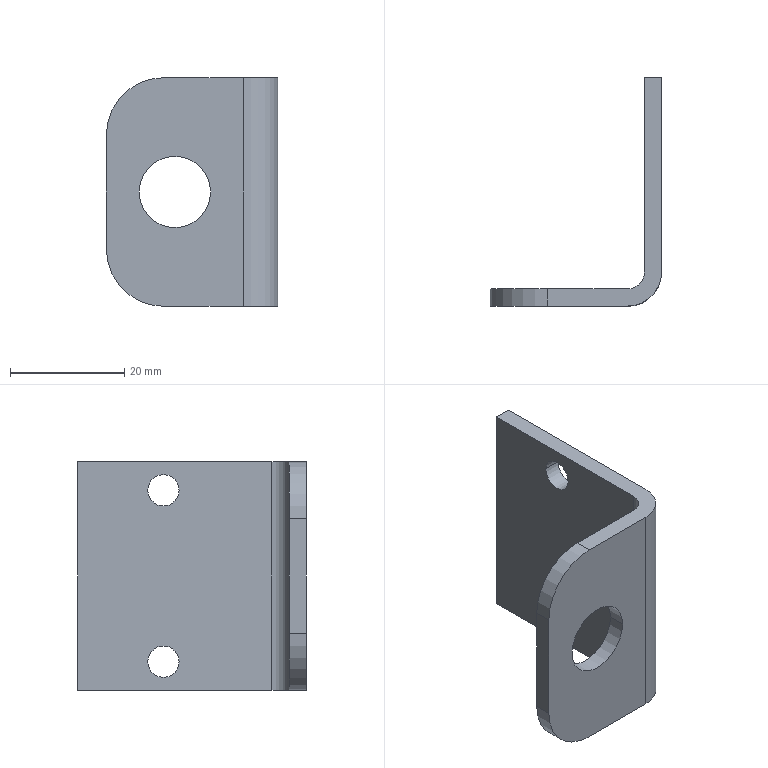Part | STEP file | X77-03025 | 1 solid | 18 faces | box 30 x 40 x 40 mm | volume 7169 mm3 | cylinder 10 | plane 8 | commonest cylinder face diameters 5.5 x4 12.5 x2 20 x2 6 x1 12 x1
STEP:
#1=CARTESIAN_POINT('',(-8.75,-40.,20.));
#2=VERTEX_POINT('',#1);
#3=CARTESIAN_POINT('',(-21.25,-40.,20.));
#4=VERTEX_POINT('',#3);
#5=CARTESIAN_POINT('',(-15.,-40.,20.));
#6=DIRECTION('',(0.,1.,0.));
#7=DIRECTION('',(-1.,0.,0.));
#8=AXIS2_PLACEMENT_3D('',#5,#6,#7);
#9=CIRCLE('',#8,6.25);
#10=EDGE_CURVE('',#2,#4,#9,.T.);
#11=ORIENTED_EDGE('',*,*,#10,.F.);
#12=CARTESIAN_POINT('',(-8.75,-37.,20.));
#13=VERTEX_POINT('',#12);
#14=CARTESIAN_POINT('',(-8.75,-40.,20.));
#15=DIRECTION('',(0.,1.,0.));
#16=VECTOR('',#15,1000.);
#17=LINE('',#14,#16);
#18=EDGE_CURVE('',#2,#13,#17,.T.);
#19=ORIENTED_EDGE('',*,*,#18,.T.);
#20=CARTESIAN_POINT('',(-21.25,-37.,20.));
#21=VERTEX_POINT('',#20);
#22=CARTESIAN_POINT('',(-15.,-37.,20.));
#23=DIRECTION('',(0.,1.,0.));
#24=DIRECTION('',(-1.,0.,0.));
#25=AXIS2_PLACEMENT_3D('',#22,#23,#24);
#26=CIRCLE('',#25,6.25);
#27=EDGE_CURVE('',#13,#21,#26,.T.);
#28=ORIENTED_EDGE('',*,*,#27,.T.);
#29=CARTESIAN_POINT('',(-21.25,-40.,20.));
#30=DIRECTION('',(0.,1.,0.));
#31=VECTOR('',#30,1000.);
#32=LINE('',#29,#31);
#33=EDGE_CURVE('',#4,#21,#32,.T.);
#34=ORIENTED_EDGE('',*,*,#33,.F.);
#35=EDGE_LOOP('',(#11,#19,#28,#34));
#36=FACE_OUTER_BOUND('',#35,.T.);
#37=CARTESIAN_POINT('',(-15.,-40.,20.));
#38=DIRECTION('',(0.,1.,0.));
#39=DIRECTION('',(-1.,0.,0.));
#40=AXIS2_PLACEMENT_3D('',#37,#38,#39);
#41=CYLINDRICAL_SURFACE('',#40,6.25);
#42=ADVANCED_FACE('',(#36),#41,.F.);
#43=CARTESIAN_POINT('',(3.,-12.25,35.));
#44=VERTEX_POINT('',#43);
#45=CARTESIAN_POINT('',(3.,-17.75,35.));
#46=VERTEX_POINT('',#45);
#47=CARTESIAN_POINT('',(3.,-15.,35.));
#48=DIRECTION('',(-1.,0.,0.));
#49=DIRECTION('',(0.,-1.,0.));
#50=AXIS2_PLACEMENT_3D('',#47,#48,#49);
#51=CIRCLE('',#50,2.75);
#52=EDGE_CURVE('',#44,#46,#51,.T.);
#53=ORIENTED_EDGE('',*,*,#52,.F.);
#54=CARTESIAN_POINT('',(0.,-12.25,35.));
#55=VERTEX_POINT('',#54);
#56=CARTESIAN_POINT('',(3.,-12.25,35.));
#57=DIRECTION('',(-1.,0.,0.));
#58=VECTOR('',#57,1000.);
#59=LINE('',#56,#58);
#60=EDGE_CURVE('',#44,#55,#59,.T.);
#61=ORIENTED_EDGE('',*,*,#60,.T.);
#62=CARTESIAN_POINT('',(0.,-17.75,35.));
#63=VERTEX_POINT('',#62);
#64=CARTESIAN_POINT('',(0.,-15.,35.));
#65=DIRECTION('',(-1.,0.,0.));
#66=DIRECTION('',(0.,-1.,0.));
#67=AXIS2_PLACEMENT_3D('',#64,#65,#66);
#68=CIRCLE('',#67,2.75);
#69=EDGE_CURVE('',#55,#63,#68,.T.);
#70=ORIENTED_EDGE('',*,*,#69,.T.);
#71=CARTESIAN_POINT('',(3.,-17.75,35.));
#72=DIRECTION('',(-1.,0.,0.));
#73=VECTOR('',#72,1000.);
#74=LINE('',#71,#73);
#75=EDGE_CURVE('',#46,#63,#74,.T.);
#76=ORIENTED_EDGE('',*,*,#75,.F.);
#77=EDGE_LOOP('',(#53,#61,#70,#76));
#78=FACE_OUTER_BOUND('',#77,.T.);
#79=CARTESIAN_POINT('',(3.,-15.,35.));
#80=DIRECTION('',(-1.,0.,0.));
#81=DIRECTION('',(0.,-1.,0.));
#82=AXIS2_PLACEMENT_3D('',#79,#80,#81);
#83=CYLINDRICAL_SURFACE('',#82,2.75);
#84=ADVANCED_FACE('',(#78),#83,.F.);
#85=CARTESIAN_POINT('',(3.,-12.25,5.));
#86=VERTEX_POINT('',#85);
#87=CARTESIAN_POINT('',(3.,-17.75,5.));
#88=VERTEX_POINT('',#87);
#89=CARTESIAN_POINT('',(3.,-15.,5.));
#90=DIRECTION('',(-1.,0.,0.));
#91=DIRECTION('',(0.,-1.,0.));
#92=AXIS2_PLACEMENT_3D('',#89,#90,#91);
#93=CIRCLE('',#92,2.75);
#94=EDGE_CURVE('',#86,#88,#93,.T.);
#95=ORIENTED_EDGE('',*,*,#94,.F.);
#96=CARTESIAN_POINT('',(0.,-12.25,5.));
#97=VERTEX_POINT('',#96);
#98=CARTESIAN_POINT('',(3.,-12.25,5.));
#99=DIRECTION('',(-1.,0.,0.));
#100=VECTOR('',#99,1000.);
#101=LINE('',#98,#100);
#102=EDGE_CURVE('',#86,#97,#101,.T.);
#103=ORIENTED_EDGE('',*,*,#102,.T.);
#104=CARTESIAN_POINT('',(0.,-17.75,5.));
#105=VERTEX_POINT('',#104);
#106=CARTESIAN_POINT('',(0.,-15.,5.));
#107=DIRECTION('',(-1.,0.,0.));
#108=DIRECTION('',(0.,-1.,0.));
#109=AXIS2_PLACEMENT_3D('',#106,#107,#108);
#110=CIRCLE('',#109,2.75);
#111=EDGE_CURVE('',#97,#105,#110,.T.);
#112=ORIENTED_EDGE('',*,*,#111,.T.);
#113=CARTESIAN_POINT('',(3.,-17.75,5.));
#114=DIRECTION('',(-1.,0.,0.));
#115=VECTOR('',#114,1000.);
#116=LINE('',#113,#115);
#117=EDGE_CURVE('',#88,#105,#116,.T.);
#118=ORIENTED_EDGE('',*,*,#117,.F.);
#119=EDGE_LOOP('',(#95,#103,#112,#118));
#120=FACE_OUTER_BOUND('',#119,.T.);
#121=CARTESIAN_POINT('',(3.,-15.,5.));
#122=DIRECTION('',(-1.,0.,0.));
#123=DIRECTION('',(0.,-1.,0.));
#124=AXIS2_PLACEMENT_3D('',#121,#122,#123);
#125=CYLINDRICAL_SURFACE('',#124,2.75);
#126=ADVANCED_FACE('',(#120),#125,.F.);
#127=CARTESIAN_POINT('',(3.,0.,0.));
#128=VERTEX_POINT('',#127);
#129=CARTESIAN_POINT('',(0.,0.,0.));
#130=VERTEX_POINT('',#129);
#131=CARTESIAN_POINT('',(3.,0.,0.));
#132=DIRECTION('',(-1.,0.,0.));
#133=VECTOR('',#132,1000.);
#134=LINE('',#131,#133);
#135=EDGE_CURVE('',#128,#130,#134,.T.);
#136=ORIENTED_EDGE('',*,*,#135,.T.);
#137=CARTESIAN_POINT('',(0.,0.,40.));
#138=VERTEX_POINT('',#137);
#139=CARTESIAN_POINT('',(0.,0.,40.));
#140=DIRECTION('',(0.,0.,-1.));
#141=VECTOR('',#140,1000.);
#142=LINE('',#139,#141);
#143=EDGE_CURVE('',#138,#130,#142,.T.);
#144=ORIENTED_EDGE('',*,*,#143,.F.);
#145=CARTESIAN_POINT('',(3.,0.,40.));
#146=VERTEX_POINT('',#145);
#147=CARTESIAN_POINT('',(3.,0.,40.));
#148=DIRECTION('',(-1.,0.,0.));
#149=VECTOR('',#148,1000.);
#150=LINE('',#147,#149);
#151=EDGE_CURVE('',#146,#138,#150,.T.);
#152=ORIENTED_EDGE('',*,*,#151,.F.);
#153=CARTESIAN_POINT('',(3.,0.,40.));
#154=DIRECTION('',(0.,0.,-1.));
#155=VECTOR('',#154,1000.);
#156=LINE('',#153,#155);
#157=EDGE_CURVE('',#146,#128,#156,.T.);
#158=ORIENTED_EDGE('',*,*,#157,.T.);
#159=EDGE_LOOP('',(#136,#144,#152,#158));
#160=FACE_OUTER_BOUND('',#159,.T.);
#161=CARTESIAN_POINT('',(3.,0.,40.));
#162=DIRECTION('',(0.,-1.,0.));
#163=DIRECTION('',(1.,0.,0.));
#164=AXIS2_PLACEMENT_3D('',#161,#162,#163);
#165=PLANE('',#164);
#166=ADVANCED_FACE('',(#160),#165,.F.);
#167=CARTESIAN_POINT('',(0.,-15.,35.));
#168=DIRECTION('',(-1.,0.,0.));
#169=DIRECTION('',(0.,-1.,0.));
#170=AXIS2_PLACEMENT_3D('',#167,#168,#169);
#171=CIRCLE('',#170,2.75);
#172=EDGE_CURVE('',#63,#55,#171,.T.);
#173=ORIENTED_EDGE('',*,*,#172,.F.);
#174=ORIENTED_EDGE('',*,*,#69,.F.);
#175=EDGE_LOOP('',(#173,#174));
#176=FACE_BOUND('',#175,.T.);
#177=CARTESIAN_POINT('',(0.,-15.,5.));
#178=DIRECTION('',(-1.,0.,0.));
#179=DIRECTION('',(0.,-1.,0.));
#180=AXIS2_PLACEMENT_3D('',#177,#178,#179);
#181=CIRCLE('',#180,2.75);
#182=EDGE_CURVE('',#105,#97,#181,.T.);
#183=ORIENTED_EDGE('',*,*,#182,.F.);
#184=ORIENTED_EDGE('',*,*,#111,.F.);
#185=EDGE_LOOP('',(#183,#184));
#186=FACE_BOUND('',#185,.T.);
#187=CARTESIAN_POINT('',(0.,-34.,0.));
#188=VERTEX_POINT('',#187);
#189=CARTESIAN_POINT('',(0.,0.,0.));
#190=DIRECTION('',(0.,-1.,0.));
#191=VECTOR('',#190,1000.);
#192=LINE('',#189,#191);
#193=EDGE_CURVE('',#130,#188,#192,.T.);
#194=ORIENTED_EDGE('',*,*,#193,.T.);
#195=CARTESIAN_POINT('',(0.,-34.,40.));
#196=VERTEX_POINT('',#195);
#197=CARTESIAN_POINT('',(0.,-34.,40.));
#198=DIRECTION('',(0.,0.,-1.));
#199=VECTOR('',#198,1000.);
#200=LINE('',#197,#199);
#201=EDGE_CURVE('',#196,#188,#200,.T.);
#202=ORIENTED_EDGE('',*,*,#201,.F.);
#203=CARTESIAN_POINT('',(0.,0.,40.));
#204=DIRECTION('',(0.,-1.,0.));
#205=VECTOR('',#204,1000.);
#206=LINE('',#203,#205);
#207=EDGE_CURVE('',#138,#196,#206,.T.);
#208=ORIENTED_EDGE('',*,*,#207,.F.);
#209=ORIENTED_EDGE('',*,*,#143,.T.);
#210=EDGE_LOOP('',(#194,#202,#208,#209));
#211=FACE_OUTER_BOUND('',#210,.T.);
#212=CARTESIAN_POINT('',(0.,0.,40.));
#213=DIRECTION('',(1.,0.,0.));
#214=DIRECTION('',(0.,1.,0.));
#215=AXIS2_PLACEMENT_3D('',#212,#213,#214);
#216=PLANE('',#215);
#217=ADVANCED_FACE('',(#176,#186,#211),#216,.F.);
#218=CARTESIAN_POINT('',(-3.,-37.,0.));
#219=VERTEX_POINT('',#218);
#220=CARTESIAN_POINT('',(-3.,-34.,0.));
#221=DIRECTION('',(0.,0.,-1.));
#222=DIRECTION('',(1.,0.,0.));
#223=AXIS2_PLACEMENT_3D('',#220,#221,#222);
#224=CIRCLE('',#223,3.);
#225=EDGE_CURVE('',#188,#219,#224,.T.);
#226=ORIENTED_EDGE('',*,*,#225,.T.);
#227=CARTESIAN_POINT('',(-3.,-37.,40.));
#228=VERTEX_POINT('',#227);
#229=CARTESIAN_POINT('',(-3.,-37.,40.));
#230=DIRECTION('',(0.,0.,-1.));
#231=VECTOR('',#230,1000.);
#232=LINE('',#229,#231);
#233=EDGE_CURVE('',#228,#219,#232,.T.);
#234=ORIENTED_EDGE('',*,*,#233,.F.);
#235=CARTESIAN_POINT('',(-3.,-34.,40.));
#236=DIRECTION('',(0.,0.,-1.));
#237=DIRECTION('',(1.,0.,0.));
#238=AXIS2_PLACEMENT_3D('',#235,#236,#237);
#239=CIRCLE('',#238,3.);
#240=EDGE_CURVE('',#196,#228,#239,.T.);
#241=ORIENTED_EDGE('',*,*,#240,.F.);
#242=ORIENTED_EDGE('',*,*,#201,.T.);
#243=EDGE_LOOP('',(#226,#234,#241,#242));
#244=FACE_OUTER_BOUND('',#243,.T.);
#245=CARTESIAN_POINT('',(-3.,-34.,40.));
#246=DIRECTION('',(0.,0.,-1.));
#247=DIRECTION('',(-1.,0.,0.));
#248=AXIS2_PLACEMENT_3D('',#245,#246,#247);
#249=CYLINDRICAL_SURFACE('',#248,3.);
#250=ADVANCED_FACE('',(#244),#249,.F.);
#251=CARTESIAN_POINT('',(-15.,-37.,20.));
#252=DIRECTION('',(0.,1.,0.));
#253=DIRECTION('',(-1.,0.,0.));
#254=AXIS2_PLACEMENT_3D('',#251,#252,#253);
#255=CIRCLE('',#254,6.25);
#256=EDGE_CURVE('',#21,#13,#255,.T.);
#257=ORIENTED_EDGE('',*,*,#256,.F.);
#258=ORIENTED_EDGE('',*,*,#27,.F.);
#259=EDGE_LOOP('',(#257,#258));
#260=FACE_BOUND('',#259,.T.);
#261=CARTESIAN_POINT('',(-27.,-37.,30.));
#262=VERTEX_POINT('',#261);
#263=CARTESIAN_POINT('',(-27.,-37.,10.));
#264=VERTEX_POINT('',#263);
#265=CARTESIAN_POINT('',(-27.,-37.,40.));
#266=DIRECTION('',(0.,0.,-1.));
#267=VECTOR('',#266,1000.);
#268=LINE('',#265,#267);
#269=EDGE_CURVE('',#262,#264,#268,.T.);
#270=ORIENTED_EDGE('',*,*,#269,.F.);
#271=CARTESIAN_POINT('',(-17.,-37.,40.));
#272=VERTEX_POINT('',#271);
#273=CARTESIAN_POINT('',(-17.,-37.,30.));
#274=DIRECTION('',(0.,1.,0.));
#275=DIRECTION('',(0.,0.,-1.));
#276=AXIS2_PLACEMENT_3D('',#273,#274,#275);
#277=CIRCLE('',#276,10.);
#278=EDGE_CURVE('',#262,#272,#277,.T.);
#279=ORIENTED_EDGE('',*,*,#278,.T.);
#280=CARTESIAN_POINT('',(-3.,-37.,40.));
#281=DIRECTION('',(-1.,0.,0.));
#282=VECTOR('',#281,1000.);
#283=LINE('',#280,#282);
#284=EDGE_CURVE('',#228,#272,#283,.T.);
#285=ORIENTED_EDGE('',*,*,#284,.F.);
#286=ORIENTED_EDGE('',*,*,#233,.T.);
#287=CARTESIAN_POINT('',(-17.,-37.,0.));
#288=VERTEX_POINT('',#287);
#289=CARTESIAN_POINT('',(-3.,-37.,0.));
#290=DIRECTION('',(-1.,0.,0.));
#291=VECTOR('',#290,1000.);
#292=LINE('',#289,#291);
#293=EDGE_CURVE('',#219,#288,#292,.T.);
#294=ORIENTED_EDGE('',*,*,#293,.T.);
#295=CARTESIAN_POINT('',(-17.,-37.,10.));
#296=DIRECTION('',(0.,1.,0.));
#297=DIRECTION('',(0.,0.,-1.));
#298=AXIS2_PLACEMENT_3D('',#295,#296,#297);
#299=CIRCLE('',#298,10.);
#300=EDGE_CURVE('',#288,#264,#299,.T.);
#301=ORIENTED_EDGE('',*,*,#300,.T.);
#302=EDGE_LOOP('',(#270,#279,#285,#286,#294,#301));
#303=FACE_OUTER_BOUND('',#302,.T.);
#304=CARTESIAN_POINT('',(-3.,-37.,40.));
#305=DIRECTION('',(0.,-1.,0.));
#306=DIRECTION('',(0.,0.,-1.));
#307=AXIS2_PLACEMENT_3D('',#304,#305,#306);
#308=PLANE('',#307);
#309=ADVANCED_FACE('',(#260,#303),#308,.F.);
#310=CARTESIAN_POINT('',(-27.,-40.,30.));
#311=VERTEX_POINT('',#310);
#312=CARTESIAN_POINT('',(-27.,-40.,10.));
#313=VERTEX_POINT('',#312);
#314=CARTESIAN_POINT('',(-27.,-40.,40.));
#315=DIRECTION('',(0.,0.,-1.));
#316=VECTOR('',#315,1000.);
#317=LINE('',#314,#316);
#318=EDGE_CURVE('',#311,#313,#317,.T.);
#319=ORIENTED_EDGE('',*,*,#318,.F.);
#320=CARTESIAN_POINT('',(-27.,-37.,30.));
#321=DIRECTION('',(0.,1.,0.));
#322=VECTOR('',#321,1000.);
#323=LINE('',#320,#322);
#324=EDGE_CURVE('',#311,#262,#323,.T.);
#325=ORIENTED_EDGE('',*,*,#324,.T.);
#326=ORIENTED_EDGE('',*,*,#269,.T.);
#327=CARTESIAN_POINT('',(-27.,-37.,10.));
#328=DIRECTION('',(0.,-1.,0.));
#329=VECTOR('',#328,1000.);
#330=LINE('',#327,#329);
#331=EDGE_CURVE('',#264,#313,#330,.T.);
#332=ORIENTED_EDGE('',*,*,#331,.T.);
#333=EDGE_LOOP('',(#319,#325,#326,#332));
#334=FACE_OUTER_BOUND('',#333,.T.);
#335=CARTESIAN_POINT('',(-27.,-37.,40.));
#336=DIRECTION('',(1.,0.,0.));
#337=DIRECTION('',(0.,1.,0.));
#338=AXIS2_PLACEMENT_3D('',#335,#336,#337);
#339=PLANE('',#338);
#340=ADVANCED_FACE('',(#334),#339,.F.);
#341=CARTESIAN_POINT('',(-15.,-40.,20.));
#342=DIRECTION('',(0.,1.,0.));
#343=DIRECTION('',(-1.,0.,0.));
#344=AXIS2_PLACEMENT_3D('',#341,#342,#343);
#345=CIRCLE('',#344,6.25);
#346=EDGE_CURVE('',#4,#2,#345,.T.);
#347=ORIENTED_EDGE('',*,*,#346,.T.);
#348=ORIENTED_EDGE('',*,*,#10,.T.);
#349=EDGE_LOOP('',(#347,#348));
#350=FACE_BOUND('',#349,.T.);
#351=CARTESIAN_POINT('',(-17.,-40.,40.));
#352=VERTEX_POINT('',#351);
#353=CARTESIAN_POINT('',(-3.,-40.,40.));
#354=VERTEX_POINT('',#353);
#355=CARTESIAN_POINT('',(-27.,-40.,40.));
#356=DIRECTION('',(1.,0.,0.));
#357=VECTOR('',#356,1000.);
#358=LINE('',#355,#357);
#359=EDGE_CURVE('',#352,#354,#358,.T.);
#360=ORIENTED_EDGE('',*,*,#359,.F.);
#361=CARTESIAN_POINT('',(-17.,-40.,30.));
#362=DIRECTION('',(0.,-1.,0.));
#363=DIRECTION('',(-1.,0.,0.));
#364=AXIS2_PLACEMENT_3D('',#361,#362,#363);
#365=CIRCLE('',#364,10.);
#366=EDGE_CURVE('',#352,#311,#365,.T.);
#367=ORIENTED_EDGE('',*,*,#366,.T.);
#368=ORIENTED_EDGE('',*,*,#318,.T.);
#369=CARTESIAN_POINT('',(-17.,-40.,0.));
#370=VERTEX_POINT('',#369);
#371=CARTESIAN_POINT('',(-17.,-40.,10.));
#372=DIRECTION('',(0.,-1.,0.));
#373=DIRECTION('',(-1.,0.,0.));
#374=AXIS2_PLACEMENT_3D('',#371,#372,#373);
#375=CIRCLE('',#374,10.);
#376=EDGE_CURVE('',#313,#370,#375,.T.);
#377=ORIENTED_EDGE('',*,*,#376,.T.);
#378=CARTESIAN_POINT('',(-3.,-40.,0.));
#379=VERTEX_POINT('',#378);
#380=CARTESIAN_POINT('',(-27.,-40.,0.));
#381=DIRECTION('',(1.,0.,0.));
#382=VECTOR('',#381,1000.);
#383=LINE('',#380,#382);
#384=EDGE_CURVE('',#370,#379,#383,.T.);
#385=ORIENTED_EDGE('',*,*,#384,.T.);
#386=CARTESIAN_POINT('',(-3.,-40.,40.));
#387=DIRECTION('',(0.,0.,-1.));
#388=VECTOR('',#387,1000.);
#389=LINE('',#386,#388);
#390=EDGE_CURVE('',#354,#379,#389,.T.);
#391=ORIENTED_EDGE('',*,*,#390,.F.);
#392=EDGE_LOOP('',(#360,#367,#368,#377,#385,#391));
#393=FACE_OUTER_BOUND('',#392,.T.);
#394=CARTESIAN_POINT('',(-27.,-40.,40.));
#395=DIRECTION('',(0.,1.,0.));
#396=DIRECTION('',(-1.,0.,0.));
#397=AXIS2_PLACEMENT_3D('',#394,#395,#396);
#398=PLANE('',#397);
#399=ADVANCED_FACE('',(#350,#393),#398,.F.);
#400=CARTESIAN_POINT('',(3.,-34.,0.));
#401=VERTEX_POINT('',#400);
#402=CARTESIAN_POINT('',(-3.,-34.,0.));
#403=DIRECTION('',(0.,0.,1.));
#404=DIRECTION('',(1.,0.,0.));
#405=AXIS2_PLACEMENT_3D('',#402,#403,#404);
#406=CIRCLE('',#405,6.);
#407=EDGE_CURVE('',#379,#401,#406,.T.);
#408=ORIENTED_EDGE('',*,*,#407,.T.);
#409=CARTESIAN_POINT('',(3.,-34.,40.));
#410=VERTEX_POINT('',#409);
#411=CARTESIAN_POINT('',(3.,-34.,40.));
#412=DIRECTION('',(0.,0.,-1.));
#413=VECTOR('',#412,1000.);
#414=LINE('',#411,#413);
#415=EDGE_CURVE('',#410,#401,#414,.T.);
#416=ORIENTED_EDGE('',*,*,#415,.F.);
#417=CARTESIAN_POINT('',(-3.,-34.,40.));
#418=DIRECTION('',(0.,0.,1.));
#419=DIRECTION('',(1.,0.,0.));
#420=AXIS2_PLACEMENT_3D('',#417,#418,#419);
#421=CIRCLE('',#420,6.);
#422=EDGE_CURVE('',#354,#410,#421,.T.);
#423=ORIENTED_EDGE('',*,*,#422,.F.);
#424=ORIENTED_EDGE('',*,*,#390,.T.);
#425=EDGE_LOOP('',(#408,#416,#423,#424));
#426=FACE_OUTER_BOUND('',#425,.T.);
#427=CARTESIAN_POINT('',(-3.,-34.,40.));
#428=DIRECTION('',(0.,0.,-1.));
#429=DIRECTION('',(-1.,0.,0.));
#430=AXIS2_PLACEMENT_3D('',#427,#428,#429);
#431=CYLINDRICAL_SURFACE('',#430,6.);
#432=ADVANCED_FACE('',(#426),#431,.T.);
#433=CARTESIAN_POINT('',(3.,-15.,35.));
#434=DIRECTION('',(-1.,0.,0.));
#435=DIRECTION('',(0.,-1.,0.));
#436=AXIS2_PLACEMENT_3D('',#433,#434,#435);
#437=CIRCLE('',#436,2.75);
#438=EDGE_CURVE('',#46,#44,#437,.T.);
#439=ORIENTED_EDGE('',*,*,#438,.T.);
#440=ORIENTED_EDGE('',*,*,#52,.T.);
#441=EDGE_LOOP('',(#439,#440));
#442=FACE_BOUND('',#441,.T.);
#443=CARTESIAN_POINT('',(3.,-15.,5.));
#444=DIRECTION('',(-1.,0.,0.));
#445=DIRECTION('',(0.,-1.,0.));
#446=AXIS2_PLACEMENT_3D('',#443,#444,#445);
#447=CIRCLE('',#446,2.75);
#448=EDGE_CURVE('',#88,#86,#447,.T.);
#449=ORIENTED_EDGE('',*,*,#448,.T.);
#450=ORIENTED_EDGE('',*,*,#94,.T.);
#451=EDGE_LOOP('',(#449,#450));
#452=FACE_BOUND('',#451,.T.);
#453=CARTESIAN_POINT('',(3.,-34.,0.));
#454=DIRECTION('',(0.,1.,0.));
#455=VECTOR('',#454,1000.);
#456=LINE('',#453,#455);
#457=EDGE_CURVE('',#401,#128,#456,.T.);
#458=ORIENTED_EDGE('',*,*,#457,.T.);
#459=ORIENTED_EDGE('',*,*,#157,.F.);
#460=CARTESIAN_POINT('',(3.,-34.,40.));
#461=DIRECTION('',(0.,1.,0.));
#462=VECTOR('',#461,1000.);
#463=LINE('',#460,#462);
#464=EDGE_CURVE('',#410,#146,#463,.T.);
#465=ORIENTED_EDGE('',*,*,#464,.F.);
#466=ORIENTED_EDGE('',*,*,#415,.T.);
#467=EDGE_LOOP('',(#458,#459,#465,#466));
#468=FACE_OUTER_BOUND('',#467,.T.);
#469=CARTESIAN_POINT('',(3.,-34.,40.));
#470=DIRECTION('',(-1.,0.,0.));
#471=DIRECTION('',(0.,0.,1.));
#472=AXIS2_PLACEMENT_3D('',#469,#470,#471);
#473=PLANE('',#472);
#474=ADVANCED_FACE('',(#442,#452,#468),#473,.F.);
#475=ORIENTED_EDGE('',*,*,#284,.T.);
#476=CARTESIAN_POINT('',(-17.,-40.,40.));
#477=DIRECTION('',(0.,-1.,0.));
#478=VECTOR('',#477,1000.);
#479=LINE('',#476,#478);
#480=EDGE_CURVE('',#272,#352,#479,.T.);
#481=ORIENTED_EDGE('',*,*,#480,.T.);
#482=ORIENTED_EDGE('',*,*,#359,.T.);
#483=ORIENTED_EDGE('',*,*,#422,.T.);
#484=ORIENTED_EDGE('',*,*,#464,.T.);
#485=ORIENTED_EDGE('',*,*,#151,.T.);
#486=ORIENTED_EDGE('',*,*,#207,.T.);
#487=ORIENTED_EDGE('',*,*,#240,.T.);
#488=EDGE_LOOP('',(#475,#481,#482,#483,#484,#485,#486,#487));
#489=FACE_OUTER_BOUND('',#488,.T.);
#490=CARTESIAN_POINT('',(-3.,-34.,40.));
#491=DIRECTION('',(0.,0.,1.));
#492=DIRECTION('',(1.,0.,0.));
#493=AXIS2_PLACEMENT_3D('',#490,#491,#492);
#494=PLANE('',#493);
#495=ADVANCED_FACE('',(#489),#494,.T.);
#496=ORIENTED_EDGE('',*,*,#384,.F.);
#497=CARTESIAN_POINT('',(-17.,-34.,0.));
#498=DIRECTION('',(0.,1.,0.));
#499=VECTOR('',#498,1000.);
#500=LINE('',#497,#499);
#501=EDGE_CURVE('',#370,#288,#500,.T.);
#502=ORIENTED_EDGE('',*,*,#501,.T.);
#503=ORIENTED_EDGE('',*,*,#293,.F.);
#504=ORIENTED_EDGE('',*,*,#225,.F.);
#505=ORIENTED_EDGE('',*,*,#193,.F.);
#506=ORIENTED_EDGE('',*,*,#135,.F.);
#507=ORIENTED_EDGE('',*,*,#457,.F.);
#508=ORIENTED_EDGE('',*,*,#407,.F.);
#509=EDGE_LOOP('',(#496,#502,#503,#504,#505,#506,#507,#508));
#510=FACE_OUTER_BOUND('',#509,.T.);
#511=CARTESIAN_POINT('',(-3.,-34.,0.));
#512=DIRECTION('',(0.,0.,1.));
#513=DIRECTION('',(1.,0.,0.));
#514=AXIS2_PLACEMENT_3D('',#511,#512,#513);
#515=PLANE('',#514);
#516=ADVANCED_FACE('',(#510),#515,.F.);
#517=ORIENTED_EDGE('',*,*,#102,.F.);
#518=ORIENTED_EDGE('',*,*,#448,.F.);
#519=ORIENTED_EDGE('',*,*,#117,.T.);
#520=ORIENTED_EDGE('',*,*,#182,.T.);
#521=EDGE_LOOP('',(#517,#518,#519,#520));
#522=FACE_OUTER_BOUND('',#521,.T.);
#523=CARTESIAN_POINT('',(3.,-15.,5.));
#524=DIRECTION('',(-1.,0.,0.));
#525=DIRECTION('',(0.,-1.,0.));
#526=AXIS2_PLACEMENT_3D('',#523,#524,#525);
#527=CYLINDRICAL_SURFACE('',#526,2.75);
#528=ADVANCED_FACE('',(#522),#527,.F.);
#529=ORIENTED_EDGE('',*,*,#60,.F.);
#530=ORIENTED_EDGE('',*,*,#438,.F.);
#531=ORIENTED_EDGE('',*,*,#75,.T.);
#532=ORIENTED_EDGE('',*,*,#172,.T.);
#533=EDGE_LOOP('',(#529,#530,#531,#532));
#534=FACE_OUTER_BOUND('',#533,.T.);
#535=CARTESIAN_POINT('',(3.,-15.,35.));
#536=DIRECTION('',(-1.,0.,0.));
#537=DIRECTION('',(0.,-1.,0.));
#538=AXIS2_PLACEMENT_3D('',#535,#536,#537);
#539=CYLINDRICAL_SURFACE('',#538,2.75);
#540=ADVANCED_FACE('',(#534),#539,.F.);
#541=ORIENTED_EDGE('',*,*,#18,.F.);
#542=ORIENTED_EDGE('',*,*,#346,.F.);
#543=ORIENTED_EDGE('',*,*,#33,.T.);
#544=ORIENTED_EDGE('',*,*,#256,.T.);
#545=EDGE_LOOP('',(#541,#542,#543,#544));
#546=FACE_OUTER_BOUND('',#545,.T.);
#547=CARTESIAN_POINT('',(-15.,-40.,20.));
#548=DIRECTION('',(0.,1.,0.));
#549=DIRECTION('',(-1.,0.,0.));
#550=AXIS2_PLACEMENT_3D('',#547,#548,#549);
#551=CYLINDRICAL_SURFACE('',#550,6.25);
#552=ADVANCED_FACE('',(#546),#551,.F.);
#553=ORIENTED_EDGE('',*,*,#278,.F.);
#554=ORIENTED_EDGE('',*,*,#324,.F.);
#555=ORIENTED_EDGE('',*,*,#366,.F.);
#556=ORIENTED_EDGE('',*,*,#480,.F.);
#557=EDGE_LOOP('',(#553,#554,#555,#556));
#558=FACE_OUTER_BOUND('',#557,.T.);
#559=CARTESIAN_POINT('',(-17.,-34.,30.));
#560=DIRECTION('',(0.,1.,0.));
#561=DIRECTION('',(-1.,0.,0.));
#562=AXIS2_PLACEMENT_3D('',#559,#560,#561);
#563=CYLINDRICAL_SURFACE('',#562,10.);
#564=ADVANCED_FACE('',(#558),#563,.T.);
#565=ORIENTED_EDGE('',*,*,#300,.F.);
#566=ORIENTED_EDGE('',*,*,#501,.F.);
#567=ORIENTED_EDGE('',*,*,#376,.F.);
#568=ORIENTED_EDGE('',*,*,#331,.F.);
#569=EDGE_LOOP('',(#565,#566,#567,#568));
#570=FACE_OUTER_BOUND('',#569,.T.);
#571=CARTESIAN_POINT('',(-17.,-37.,10.));
#572=DIRECTION('',(0.,-1.,0.));
#573=DIRECTION('',(1.,0.,0.));
#574=AXIS2_PLACEMENT_3D('',#571,#572,#573);
#575=CYLINDRICAL_SURFACE('',#574,10.);
#576=ADVANCED_FACE('',(#570),#575,.T.);
#577=CLOSED_SHELL('',(#42,#84,#126,#166,#217,#250,#309,#340,#399,#432,#474,#495,#516,#528,#540,#552,#564,#576));
#578=MANIFOLD_SOLID_BREP('',#577);
#579=CARTESIAN_POINT('',(0.,0.,0.));
#580=DIRECTION('',(0.,0.,1.));
#581=DIRECTION('',(1.,0.,0.));
#582=AXIS2_PLACEMENT_3D('',#579,#580,#581);
#583=(LENGTH_UNIT()NAMED_UNIT(*)SI_UNIT(.MILLI.,.METRE.));
#584=UNCERTAINTY_MEASURE_WITH_UNIT(LENGTH_MEASURE(0.00001),#583,'','');
#585=(NAMED_UNIT(*)PLANE_ANGLE_UNIT()SI_UNIT($,.RADIAN.));
#586=(NAMED_UNIT(*)SI_UNIT($,.STERADIAN.)SOLID_ANGLE_UNIT());
#587=(GEOMETRIC_REPRESENTATION_CONTEXT(3)GLOBAL_UNCERTAINTY_ASSIGNED_CONTEXT((#584))GLOBAL_UNIT_ASSIGNED_CONTEXT((#583,#585,#586))REPRESENTATION_CONTEXT('',''));
#588=ADVANCED_BREP_SHAPE_REPRESENTATION('',(#578,#582),#587);